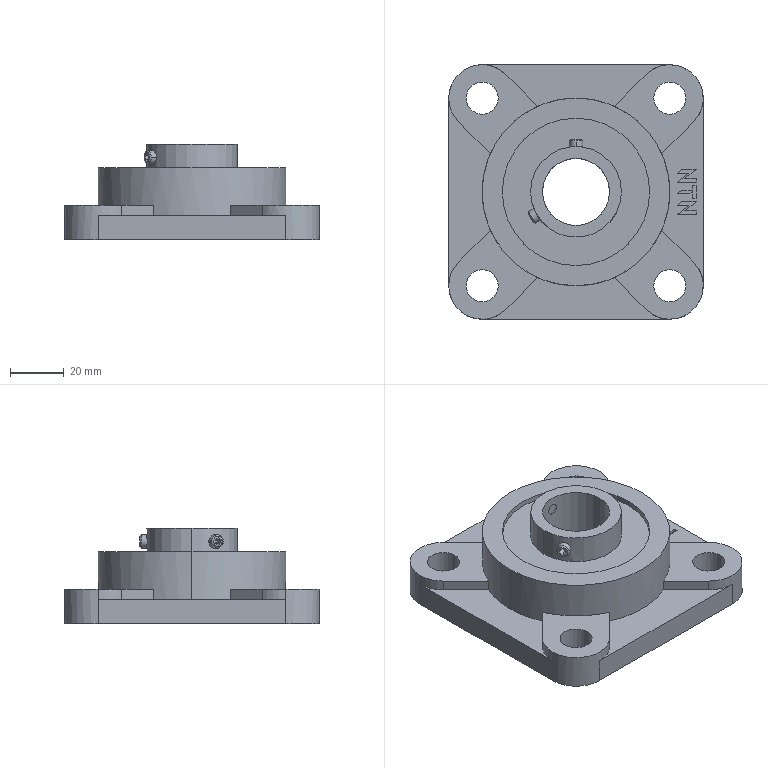Part | STEP file | _UCF205 HOUSING.stp | 1 solid | 126 faces | box 95 x 95 x 35.8 mm | volume 112730 mm3 | plane 81 | cylinder 41 | cone 4 | commonest cylinder face diameters 25 x14 12 x8 4.019 x5 5 x4 33.9 x4 55 x4